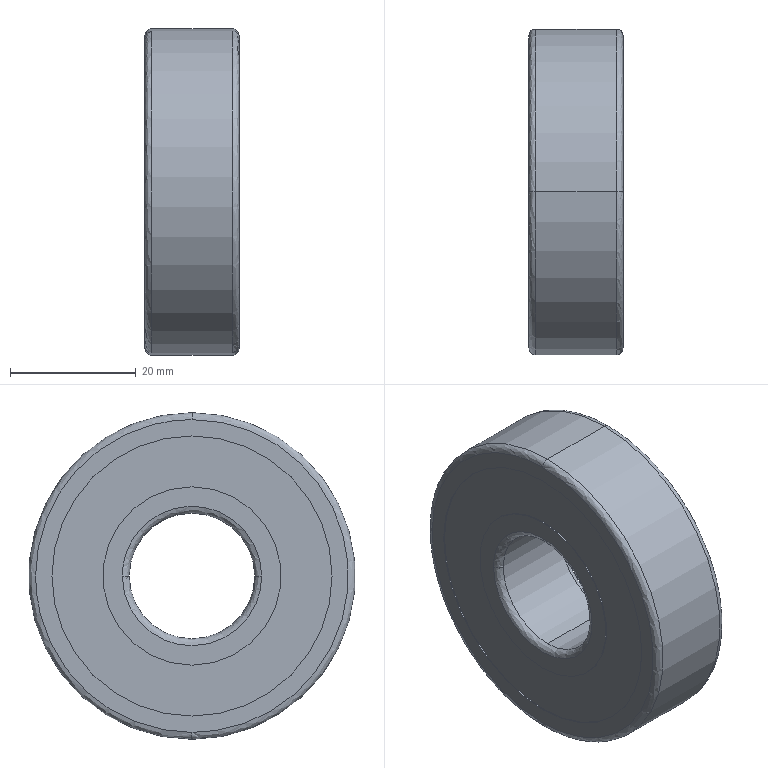Part | SolidWorks | features BaseBody 13 | 13 solids | 72 faces | box 15 x 52 x 52 mm | volume 19134 mm3 | spline 32 | cylinder 28 | plane 12 | commonest cylinder face diameters 28.4 x8 44.6 x8 30.2 x4 42 x4 20 x2 52 x2